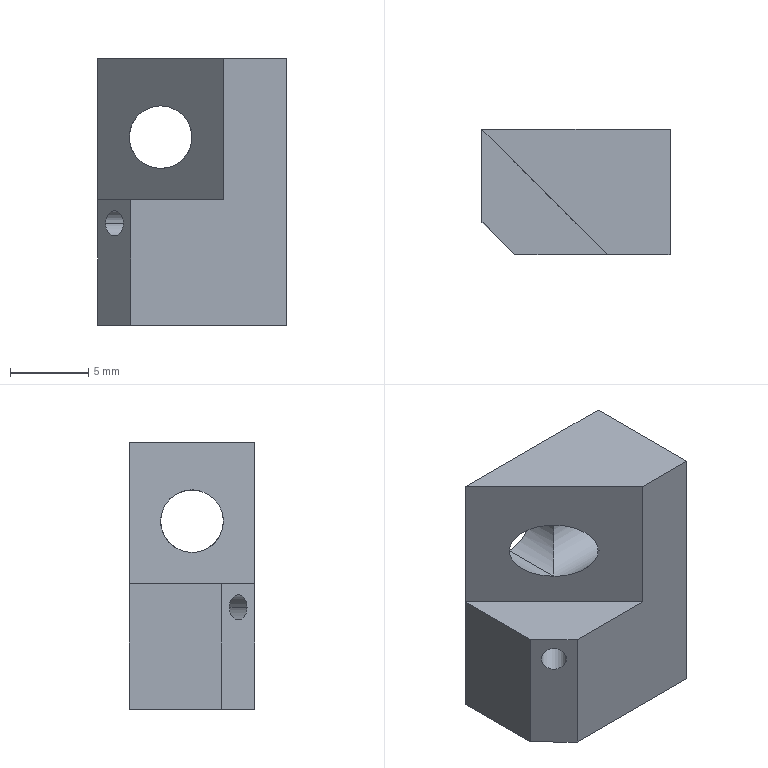NC program | NX | posted with a generic post | part box 12 x 8 x 17 mm
Whole program:
N10 G17 G21 G94 G90
(DRILLING , TOOL : D6A45)
N12 T07 M6
N14 G54
N16 G17 G0 G90 X0. Y2.5 S5000 M3
N18 G43 Z30. H7
N20 G94 G81 G98 Z-0.9 F250. R3.
N22 X-4. Y0.
N24 X0. Y-2.5
N26 X4. Y0.
N28 G80
N30 G0 X4. Y0. Z30.
N32 M5
(DRILLING_COPY_COPY , TOOL : 1.6ZT)
N34 T14 M6
N36 G54
N38 G17 G0 G90 X4. Y0. S2000 M3
N40 G43 Z30. H14
N42 G94 G83 G98 Z-5.2 F150. Q2. R3.
N44 X0. Y2.5 Z-3.88
N46 X-4. Y0. Z-5.2
N48 X0. Y-2.5 Z-3.88
N50 G80
N52 G0 X0. Y-2.5 Z30.
N54 M5
(HOLE_MILLING , TOOL : D1.)
N56 T01 M6
N58 G54
N60 G17 G0 G90 X0. Y2.5 S9500 M3
N62 G43 Z30. H1
N64 Z0.5
N66 G94 G3 X-0.225 Y2.725 R0.225 F1000.
N68 X-0.45 Y2.5 R0.225
N70 X-0.45 Y2.5 Z0.42 I0.45 J0.
N72 X-0.45 Y2.5 Z0.34 I0.45 J0.
N74 X-0.45 Y2.5 Z0.26 I0.45 J0.
N76 X-0.45 Y2.5 Z0.18 I0.45 J0.
N78 X-0.45 Y2.5 Z0.1 I0.45 J0.
N80 X-0.45 Y2.5 Z0.02 I0.45 J0.
N82 X-0.45 Y2.5 Z-0.06 I0.45 J0.
N84 X-0.45 Y2.5 Z-0.14 I0.45 J0.
N86 X-0.45 Y2.5 Z-0.22 I0.45 J0.
N88 X-0.45 Y2.5 Z-0.3 I0.45 J0.
N90 X-0.45 Y2.5 Z-0.38 I0.45 J0.
N92 X-0.45 Y2.5 Z-0.46 I0.45 J0.
N94 X-0.45 Y2.5 Z-0.54 I0.45 J0.
N96 X-0.45 Y2.5 Z-0.62 I0.45 J0.
N98 X-0.45 Y2.5 Z-0.7 I0.45 J0.
N100 X-0.45 Y2.5 Z-0.78 I0.45 J0.
N102 X-0.45 Y2.5 Z-0.86 I0.45 J0.
N104 X-0.45 Y2.5 Z-0.94 I0.45 J0.
N106 X-0.45 Y2.5 Z-1.02 I0.45 J0.
N108 X-0.45 Y2.5 Z-1.1 I0.45 J0.
N110 X-0.45 Y2.5 Z-1.18 I0.45 J0.
N112 X-0.45 Y2.5 Z-1.26 I0.45 J0.
N114 X-0.45 Y2.5 Z-1.34 I0.45 J0.
N116 X-0.45 Y2.5 Z-1.42 I0.45 J0.
N118 X-0.45 Y2.5 Z-1.5 I0.45 J0.
N120 X-0.45 Y2.5 Z-1.58 I0.45 J0.
N122 X-0.45 Y2.5 Z-1.66 I0.45 J0.
N124 X-0.45 Y2.5 Z-1.74 I0.45 J0.
N126 X-0.45 Y2.5 Z-1.82 I0.45 J0.
N128 X-0.45 Y2.5 Z-1.9 I0.45 J0.
N130 X-0.45 Y2.5 Z-1.98 I0.45 J0.
N132 X-0.45 Y2.5 Z-2.06 I0.45 J0.
N134 X-0.45 Y2.5 Z-2.14 I0.45 J0.
N136 X-0.45 Y2.5 Z-2.22 I0.45 J0.
N138 X-0.45 Y2.5 Z-2.3 I0.45 J0.
N140 X-0.45 Y2.5 Z-2.38 I0.45 J0.
N142 X-0.45 Y2.5 Z-2.46 I0.45 J0.
N144 X-0.45 Y2.5 Z-2.54 I0.45 J0.
N146 X-0.45 Y2.5 Z-2.62 I0.45 J0.
N148 X-0.45 Y2.5 Z-2.7 I0.45 J0.
N150 X-0.45 Y2.5 Z-2.78 I0.45 J0.
N152 X-0.45 Y2.5 Z-2.86 I0.45 J0.
N154 X-0.45 Y2.5 Z-2.94 I0.45 J0.
N156 X-0.45 Y2.5 Z-3.02 I0.45 J0.
N158 X-0.45 Y2.5 Z-3.1 I0.45 J0.
N160 X-0.45 Y2.5 Z-3.18 I0.45 J0.
N162 X-0.45 Y2.5 Z-3.26 I0.45 J0.
N164 X-0.45 Y2.5 Z-3.34 I0.45 J0.
N166 X0.03 Y2.949 Z-3.399 R-0.45
N168 X-0.449 Y2.53 R0.45
N170 X0.03 Y2.949 R-0.45
N172 X-0.209 Y2.74 R0.225
N174 X0. Y2.5 R0.225
N176 G0 Z30.
N178 Y-2.5
N180 Z0.5
N182 G3 X-0.225 Y-2.275 R0.225
N184 X-0.45 Y-2.5 R0.225
N186 X-0.45 Y-2.5 Z0.42 I0.45 J0.
N188 X-0.45 Y-2.5 Z0.34 I0.45 J0.
N190 X-0.45 Y-2.5 Z0.26 I0.45 J0.
N192 X-0.45 Y-2.5 Z0.18 I0.45 J0.
N194 X-0.45 Y-2.5 Z0.1 I0.45 J0.
N196 X-0.45 Y-2.5 Z0.02 I0.45 J0.
N198 X-0.45 Y-2.5 Z-0.06 I0.45 J0.
N200 X-0.45 Y-2.5 Z-0.14 I0.45 J0.
N202 X-0.45 Y-2.5 Z-0.22 I0.45 J0.
N204 X-0.45 Y-2.5 Z-0.3 I0.45 J0.
N206 X-0.45 Y-2.5 Z-0.38 I0.45 J0.
N208 X-0.45 Y-2.5 Z-0.46 I0.45 J0.
N210 X-0.45 Y-2.5 Z-0.54 I0.45 J0.
N212 X-0.45 Y-2.5 Z-0.62 I0.45 J0.
N214 X-0.45 Y-2.5 Z-0.7 I0.45 J0.
N216 X-0.45 Y-2.5 Z-0.78 I0.45 J0.
N218 X-0.45 Y-2.5 Z-0.86 I0.45 J0.
N220 X-0.45 Y-2.5 Z-0.94 I0.45 J0.
N222 X-0.45 Y-2.5 Z-1.02 I0.45 J0.
N224 X-0.45 Y-2.5 Z-1.1 I0.45 J0.
N226 X-0.45 Y-2.5 Z-1.18 I0.45 J0.
N228 X-0.45 Y-2.5 Z-1.26 I0.45 J0.
N230 X-0.45 Y-2.5 Z-1.34 I0.45 J0.
N232 X-0.45 Y-2.5 Z-1.42 I0.45 J0.
N234 X-0.45 Y-2.5 Z-1.5 I0.45 J0.
N236 X-0.45 Y-2.5 Z-1.58 I0.45 J0.
N238 X-0.45 Y-2.5 Z-1.66 I0.45 J0.
N240 X-0.45 Y-2.5 Z-1.74 I0.45 J0.
N242 X-0.45 Y-2.5 Z-1.82 I0.45 J0.
N244 X-0.45 Y-2.5 Z-1.9 I0.45 J0.
N246 X-0.45 Y-2.5 Z-1.98 I0.45 J0.
N248 X-0.45 Y-2.5 Z-2.06 I0.45 J0.
N250 X-0.45 Y-2.5 Z-2.14 I0.45 J0.
N252 X-0.45 Y-2.5 Z-2.22 I0.45 J0.
N254 X-0.45 Y-2.5 Z-2.3 I0.45 J0.
N256 X-0.45 Y-2.5 Z-2.38 I0.45 J0.
N258 X-0.45 Y-2.5 Z-2.46 I0.45 J0.
N260 X-0.45 Y-2.5 Z-2.54 I0.45 J0.
N262 X-0.45 Y-2.5 Z-2.62 I0.45 J0.
N264 X-0.45 Y-2.5 Z-2.7 I0.45 J0.
N266 X-0.45 Y-2.5 Z-2.78 I0.45 J0.
N268 X-0.45 Y-2.5 Z-2.86 I0.45 J0.
N270 X-0.45 Y-2.5 Z-2.94 I0.45 J0.
N272 X-0.45 Y-2.5 Z-3.02 I0.45 J0.
N274 X-0.45 Y-2.5 Z-3.1 I0.45 J0.
N276 X-0.45 Y-2.5 Z-3.18 I0.45 J0.
N278 X-0.45 Y-2.5 Z-3.26 I0.45 J0.
N280 X-0.45 Y-2.5 Z-3.34 I0.45 J0.
N282 X0.03 Y-2.051 Z-3.399 R-0.45
N284 X-0.449 Y-2.47 R0.45
N286 X0.03 Y-2.051 R-0.45
N288 X-0.209 Y-2.26 R0.225
N290 X0. Y-2.5 R0.225
N292 G0 Z30.
N294 M5
(DRILLING_COPY , TOOL : D6A45)
N296 T07 M6
N298 G54
N300 G17 G0 G90 X0. Y2.5 S5000 M3
N302 G43 Z30. H7
N304 G94 G81 G98 Z-1.1 F250. R3.
N306 Y-2.5
N308 G80
N310 G0 X0. Y-2.5 Z30.
N312 M5
(刀补1 , TOOL : D1.)
N314 T01 M6
N316 G54
N318 G17 G0 G90 X0. Y2.5 S9500 M3
N320 G43 Z30. H1
N322 Z0.5
N324 G41 G94 G1 X-0.026 Y2.597 F850. D1
N326 G3 X-0.46 Y2.5 R0.228
N328 X-0.46 Y2.5 Z-0.5 I0.46 J0.
N330 X-0.46 Y2.5 Z-1.5 I0.46 J0.
N332 X-0.46 Y2.5 Z-2.5 I0.46 J0.
N334 X-0.371 Y2.772 Z-3.399 R-0.46
N336 X-0.272 Y2.129 R0.46
N338 X-0.371 Y2.772 R-0.46
N340 X-0.078 Y2.438 R0.228
N342 G40
N344 G1 X0. Y2.5
N346 G0 Z30.
N348 Y-2.5
N350 Z0.5
N352 G41 G1 X-0.026 Y-2.403
N354 G3 X-0.46 Y-2.5 R0.228
N356 X-0.46 Y-2.5 Z-0.5 I0.46 J0.
N358 X-0.46 Y-2.5 Z-1.5 I0.46 J0.
N360 X-0.46 Y-2.5 Z-2.5 I0.46 J0.
N362 X-0.371 Y-2.228 Z-3.399 R-0.46
N364 X-0.272 Y-2.871 R0.46
N366 X-0.371 Y-2.228 R-0.46
N368 X-0.078 Y-2.562 R0.228
N370 G40
N372 G1 X0. Y-2.5
N374 G0 Z30.
N376 M5
N378 M2